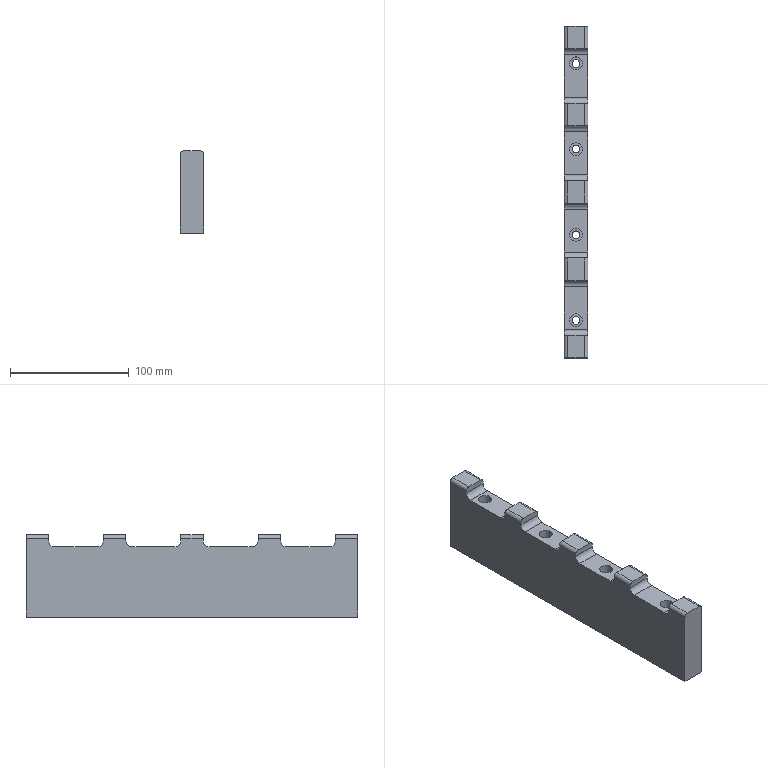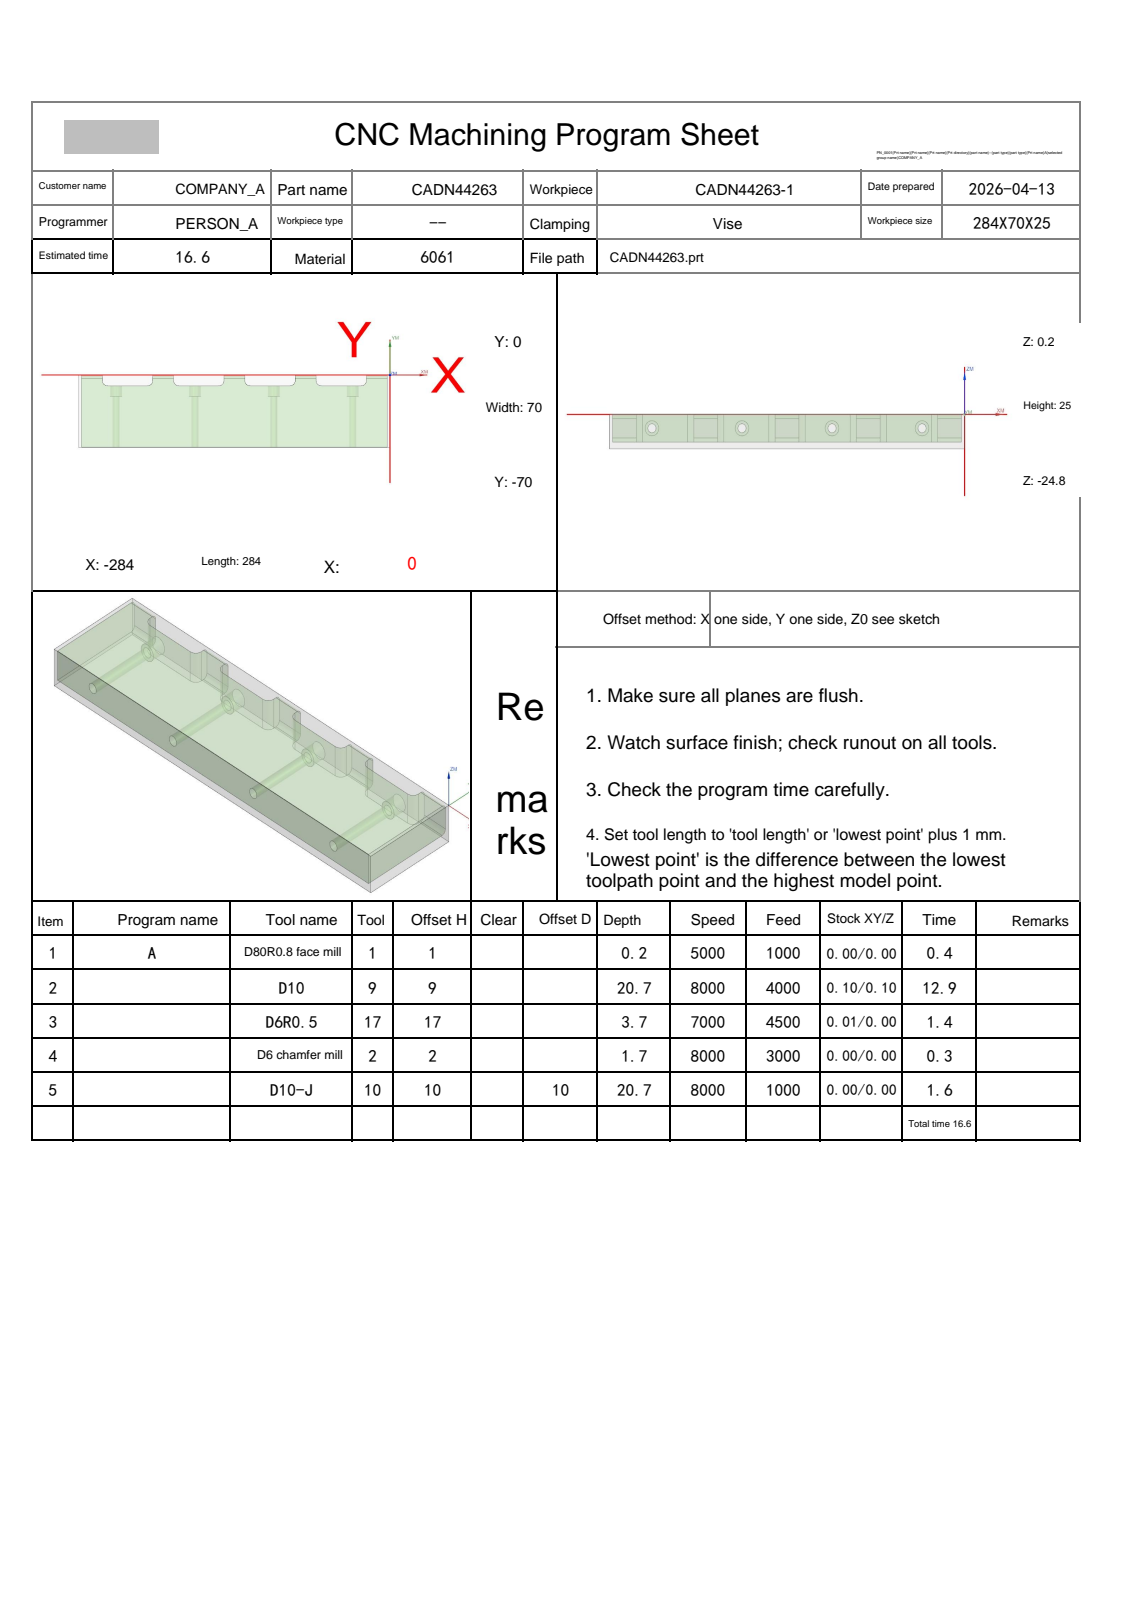NC program | NX | posted by the shop | part box 20 x 279 x 69 mm
Lines 7914 to 9859 of 9859:
N3 T17 M06
(D6R0.5  D=6. R=0.5 H=17 ce=0.01 di=0.00)
G00 G90 G54 X-27.305 Y-.497 M03 S7000
G43 H17 Z10.2
M08
Z.493
G01 Z-.007 F4500.
X-22.6 Y-.968
X-22.418 Y-.967
X-21.5 Y-.762
X-2.5
G03 X-1.496 Y-.906 I1.004 J3.433
G01 X-1.377 Y-.904
X-1.388 Y-.838 Z-.015
G03 X-2.5 Y-.667 I-1.295 J-4.708
G01 X-21.5
X-22.6 Y-.861
Y-.779 Z-.019
Y-.748 Z-.023
X-22.38 Y-.732
X-21.5 Y-.59
X-2.5
X-1.397 Y-.771
X-1.4 Y-.71 Z-.032
G03 X-2.5 Y-.521 I-3.068 J-14.528
G01 X-21.5
X-22.418 Y-.687
X-22.6 Y-.688
Y-.639 Z-.037
Y-.627 Z-.042
X-21.5 Y-.447
X-2.5
G02 X-1.4 Y-.653 I-2.113 J-14.314
G01 Y-.602 Z-.049
Y-.587 Z-.055
X-1.608 Y-.53
X-2.5 Y-.372
X-21.5
X-22.6 Y-.554
Y-.493 Z-.062
Y-.472 Z-.069
X-21.5 Y-.297
X-2.5
G02 X-1.4 Y-.511 I-.298 J-4.464
G01 Y-.425 Z-.086
X-2.5 Y-.221
X-21.5
X-22.6 Y-.382
Y-.345 Z-.095
Y-.314 Z-.104
X-21.5 Y-.143
X-2.5
X-1.4 Y-.343
Y-.304 Z-.114
Y-.258 Z-.125
X-2.5 Y-.063
X-21.5
X-22.6 Y-.235
Y-.189 Z-.137
Y-.148 Z-.148
X-21.5 Y.018
X-2.5
G02 X-1.4 Y-.164 I-.51 J-6.477
G01 Y-.114 Z-.161
Y-.062 Z-.174
X-1.576 Y-.054
X-1.673 Y-.027
X-2.5 Y.099
X-21.5
X-22.6 Y-.053
Y.003 Z-.188
Y.044 Z-.203
X-21.5 Y.184
X-2.5
G03 X-1.399 Y.042 I9.198 J66.835
G01 Y.095 Z-.219
X-1.398 Y.144 Z-.235
G02 X-2.5 Y.27 I.451 J8.779
G01 X-21.5
X-22.6 Y.142
Y.186 Z-.252
Y.225 Z-.269
X-21.5 Y.356
X-2.5
X-1.912 Y.291
X-1.826 Y.267
X-1.399 Y.227
X-1.4 Y.272 Z-.288
Y.314 Z-.306
X-2.5 Y.442
X-21.5
X-22.418 Y.317
X-22.6 Y.314
Y.354 Z-.321
Y.384 Z-.337
G03 X-21.5 Y.507 I-11.808 J110.237
G01 X-2.5
G03 X-1.4 Y.383 I2.105 J13.666
G01 Y.436 Z-.355
Y.467 Z-.374
G02 X-2.5 Y.584 I.826 J12.997
G01 X-21.5
X-22.418 Y.478
X-22.6 Y.47
Y.532 Z-.396
Y.566 Z-.418
X-22.418 Y.572
X-21.5 Y.669
X-2.5
G03 X-1.4 Y.567 I1.918 J14.664
G01 Y.619 Z-.442
Y.661 Z-.465
G02 X-2.5 Y.753 I.149 J8.39
G01 X-21.5
X-22.418 Y.662
X-22.6 Y.66
Y.702 Z-.49
Y.74 Z-.515
X-22.418 Y.743
X-21.5 Y.837
X-2.5
G03 X-1.4 Y.742 I1.224 J7.766
G01 Y.785 Z-.54
Y.826 Z-.566
G02 X-2.5 Y.918 I.174 J8.658
G01 X-21.5
X-22.418 Y.827
X-22.6 Y.824
Y.868 Z-.591
Y.907 Z-.617
X-22.418 Y.91
X-21.5 Y.995
X-2.5
G02 X-1.758 Y.91 I-.148 J-4.592
G01 X-1.4 Y.909
Y.953 Z-.644
Y.99 Z-.67
G02 X-2.5 Y1.069 I.078 J8.763
G01 X-21.5
X-22.418 Y.991
X-22.6 Y.989
Y1.037 Z-.699
Y1.062 Z-.729
X-22.418 Y1.064
X-21.5 Y1.148
X-2.5
G03 X-1.4 Y1.063 I1.15 J7.772
G01 Y1.114 Z-.759
Y1.139 Z-.79
G02 X-2.5 Y1.225 I.077 J8.113
G01 X-21.5
G02 X-22.6 Y1.138 I-1.349 J10.062
G01 Y1.187 Z-.822
Y1.216 Z-.853
G03 X-21.5 Y1.3 I-.451 J13.214
G01 X-2.5
G03 X-1.4 Y1.218 I1.277 J9.723
G01 Y1.263 Z-.886
Y1.3 Z-.919
G02 X-2.5 Y1.374 I.219 J11.451
G01 X-21.5
G02 X-22.6 Y1.298 I-1.629 J15.613
G01 Y1.341 Z-.952
Y1.374 Z-.986
G03 X-21.5 Y1.445 I-.337 J13.725
G01 X-2.5
G03 X-1.4 Y1.376 I1.224 J10.625
G01 X-1.399 Y1.419 Z-1.021
Y1.453 Z-1.056
G02 X-2.5 Y1.515 I.127 J11.964
G01 X-21.5
G02 X-22.6 Y1.451 I-1.481 J15.85
G01 Y1.489 Z-1.092
Y1.52 Z-1.128
G03 X-21.5 Y1.584 I-.16 J12.289
G01 X-2.5
G03 X-1.399 Y1.521 I1.136 J10.344
G01 Y1.554 Z-1.165
X-1.4 Y1.585 Z-1.202
G02 X-2.5 Y1.65 I.093 J10.893
G01 X-21.5
G03 X-22.073 Y1.596 I.041 J-3.531
G01 X-22.6 Y1.583
Y1.618 Z-1.24
Y1.648 Z-1.278
X-22.073 Y1.661
G02 X-21.5 Y1.714 I.679 J-4.208
G01 X-2.5
G03 X-1.4 Y1.649 I1.189 J10.851
G01 Y1.683 Z-1.316
Y1.713 Z-1.355
G02 X-2.5 Y1.776 I.065 J10.868
G01 X-21.5
G02 X-22.6 Y1.712 I-1.413 J14.76
G01 Y1.75 Z-1.395
Y1.777 Z-1.434
G03 X-21.5 Y1.836 I-.604 J21.629
G01 X-2.5
G03 X-1.399 Y1.779 I1.204 J12.62
G01 Y1.81 Z-1.475
Y1.84 Z-1.516
X-1.42
G02 X-2.5 Y1.893 I0.0 J11.063
G01 X-21.5
G02 X-22.6 Y1.839 I-1.187 J12.876
G01 Y1.867 Z-1.557
Y1.89 Z-1.598
X-22.073 Y1.9
X-21.5 Y1.948
X-2.5
G03 X-1.412 Y1.891 I1.088 J10.306
G01 X-1.399
Y1.918 Z-1.641
X-1.4 Y1.943 Z-1.683
X-1.562 Y1.938
G02 X-1.773 Y1.946 I0.0 J2.647
G01 X-2.447 Y2.
X-2.5 Y2.001
X-21.5
G03 X-22.073 Y1.952 I.057 J-4.043
G01 X-22.6 Y1.941
Y1.97 Z-1.726
Y1.996 Z-1.769
X-22.073 Y2.005
G02 X-21.5 Y2.052 I.847 J-6.832
G01 X-2.5
G03 X-1.446 Y1.996 I1.054 J9.941
G01 X-1.4
Y2.023 Z-1.812
X-1.399 Y2.049 Z-1.856
X-1.52 Y2.048
G02 X-2.5 Y2.1 I0.0 J9.293
G01 X-21.5
G02 X-22.6 Y2.047 I-1.179 J13.117
G01 Y2.073 Z-1.9
Y2.096 Z-1.945
G03 X-21.5 Y2.145 I-.089 J14.098
G01 X-2.5
G03 X-1.528 Y2.096 I.972 J9.5
G01 X-1.399 Y2.097
Y2.118 Z-1.99
Y2.136 Z-2.035
X-1.411
G02 X-2.5 Y2.189 I0.0 J11.318
G01 X-21.5
G03 X-22.073 Y2.144 I.096 J-4.959
G01 X-22.6 Y2.135
Y2.157 Z-2.08
Y2.174 Z-2.126
X-22.073 Y2.183
G02 X-21.5 Y2.229 I.696 J-5.119
G01 X-2.5
G03 X-1.42 Y2.175 I1.08 J10.819
G01 X-1.399
Y2.195 Z-2.172
Y2.214 Z-2.218
X-1.403
G02 X-2.5 Y2.267 I0.0 J11.287
G01 X-21.5
G03 X-22.073 Y2.222 I.075 J-4.597
G01 X-22.6 Y2.212
Y2.234 Z-2.265
Y2.251 Z-2.312
X-22.073 Y2.259
G02 X-21.5 Y2.302 I.781 J-6.53
G01 X-2.5
G03 X-1.458 Y2.252 I1.041 J10.8
G01 X-1.399
Y2.271 Z-2.359
Y2.291 Z-2.406
X-1.511 Y2.29
G02 X-2.5 Y2.335 I0.0 J10.989
G01 X-21.5
G03 X-22.073 Y2.291 I.123 J-5.442
G01 X-22.6 Y2.289
Y2.308 Z-2.454
Y2.316 Z-2.502
X-22.073 Y2.324
X-21.5 Y2.365
X-2.5
G03 X-1.448 Y2.318 I1.052 J11.969
G01 X-1.4 Y2.319
Y2.333 Z-2.55
Y2.346 Z-2.598
X-1.538 Y2.345
G02 X-2.5 Y2.392 I0.0 J9.984
G01 X-21.5
G02 X-22.604 Y2.343 I-1.132 J13.014
G01 Y2.354 Z-2.646
Y2.366 Z-2.695
G03 X-21.5 Y2.416 I-.184 J16.282
G01 X-2.5
G03 X-1.557 Y2.371 I.943 J9.825
G01 X-1.405 Y2.372
X-1.404 Y2.385 Z-2.744
Y2.398 Z-2.792
X-1.564 Y2.397
G02 X-2.5 Y2.438 I0.0 J10.791
G01 X-21.5
G02 X-22.604 Y2.39 I-1.539 J22.701
G01 X-22.605 Y2.401 Z-2.841
Y2.413 Z-2.891
G03 X-21.5 Y2.457 I-.624 J29.922
G01 X-2.5
G03 X-1.538 Y2.424 I.962 J14.016
G01 X-1.402
Y2.431 Z-2.94
X-1.401 Y2.444 Z-2.989
X-1.586 Y2.443
G02 X-2.5 Y2.473 I0.0 J14.194
G01 X-21.5
G02 X-22.605 Y2.434 I-1.958 J40.051
G01 Y2.444 Z-3.039
Y2.454 Z-3.088
X-21.5 Y2.486
X-2.5
G03 X-1.634 Y2.461 I.866 J14.975
X-1.4 Y2.463 I0.0 J15.
G01 Y2.471 Z-3.138
Y2.476 Z-3.188
G02 X-1.643 Y2.475 I-.243 J17.246
X-2.5 Y2.496 I0.0 J17.248
G01 X-21.5
G02 X-22.459 Y2.473 I-.959 J19.531
G01 X-22.6
X-22.595 Y2.483 Z-3.266
X-22.411 Y2.482
G03 X-21.5 Y2.502 I0.0 J20.891
G01 X-2.5
X-2.447 Y2.498
X-1.399 Y2.486
Y2.495 Z-3.344
X-2.5 Y2.507
X-21.5
G02 X-22.383 Y2.492 I-.883 J27.323
G01 X-22.595 Y2.493
Y2.503 Z-3.422
X-21.5 Y2.509
X-2.5
X-1.398 Y2.504
Y2.509 Z-3.5
X-22.595 Y2.51
G00 Z10.2
X-92.277 Y-.467
Z.493
G01 Z-.007
X-87.6 Y-.968
X-87.382 Y-.967
X-86.5 Y-.762
X-67.5
X-66.618 Y-.967
X-66.41 Y-.927
X-66.403 Y-.862 Z-.011
X-66.402 Y-.849 Z-.015
X-67.31 Y-.693
X-67.5 Y-.667
X-86.5
G02 X-87.6 Y-.86 I-11.743 J63.548
G01 Y-.779 Z-.019
Y-.748 Z-.023
X-86.5 Y-.59
X-67.5
X-66.398 Y-.768
X-66.4 Y-.71 Z-.032
X-66.613 Y-.682
X-67.5 Y-.521
X-86.5
X-87.382 Y-.687
X-87.6 Y-.688
Y-.639 Z-.037
Y-.625 Z-.042
X-87.382 Y-.623
X-86.5 Y-.447
X-67.5
X-66.609 Y-.607
X-66.4 Y-.653
Y-.602 Z-.049
Y-.585 Z-.055
X-66.596 Y-.545
X-67.5 Y-.372
X-86.5
X-87.382 Y-.549
X-87.6 Y-.552
Y-.493 Z-.062
Y-.469 Z-.069
X-86.5 Y-.297
X-67.5
G02 X-66.4 Y-.508 I-1.243 J-9.475
G01 Y-.457 Z-.077
Y-.419 Z-.086
X-66.566 Y-.393
X-67.5 Y-.221
X-86.5
X-87.6 Y-.38
Y-.345 Z-.095
Y-.311 Z-.104
X-86.5 Y-.143
X-67.5
X-66.445 Y-.33
Y-.302 Z-.114
Y-.247 Z-.125
X-67.5 Y-.063
X-86.5
X-87.6 Y-.232
Y-.189 Z-.137
Y-.145 Z-.148
X-86.5 Y.018
X-67.5
X-67.31 Y.003
X-66.445 Y-.154
X-66.439 Y-.114 Z-.161
X-66.43 Y-.057 Z-.174
X-67.5 Y.099
X-86.5
X-87.6 Y-.05
Y.003 Z-.188
Y.046 Z-.203
X-87.382 Y.05
X-86.5 Y.184
X-67.5
X-66.618 Y.05
X-66.399 Y.043
X-66.4 Y.096 Z-.219
Y.143 Z-.235
X-67.5 Y.27
X-86.5
X-87.382 Y.145
X-87.6 Y.143
Y.186 Z-.252
Y.226 Z-.269
X-87.382 Y.228
X-86.5 Y.356
X-67.5
X-66.4 Y.226
Y.272 Z-.288
Y.313 Z-.306
X-66.618 Y.315
X-67.5 Y.442
X-86.5
X-87.382 Y.317
X-87.6 Y.314
Y.354 Z-.321
Y.384 Z-.337
G03 X-86.5 Y.507 I-11.318 J105.893
G01 X-67.5
X-66.618 Y.384
X-66.4 Y.382
Y.436 Z-.355
Y.466 Z-.374
X-67.5 Y.584
X-86.5
X-87.382 Y.478
X-87.6 Y.47
Y.533 Z-.396
Y.567 Z-.418
X-87.131 Y.6
X-87.036 Y.617
G02 X-86.5 Y.669 I.598 J-3.336
G01 X-67.5
X-66.4 Y.565
Y.619 Z-.442
Y.66 Z-.465
X-66.618 Y.662
X-67.5 Y.753
X-86.5
G02 X-87.6 Y.66 I-1.695 J13.465
G01 Y.702 Z-.49
Y.741 Z-.515
G03 X-86.5 Y.837 I-.518 J12.298
G01 X-67.5
G02 X-66.792 Y.747 I-.042 J-3.181
G01 X-66.4 Y.741
Y.785 Z-.54
Y.825 Z-.566
X-66.618 Y.827
X-67.5 Y.918
X-86.5
G02 X-87.6 Y.825 I-1.556 J11.791
G01 Y.868 Z-.591
Y.908 Z-.617
X-87.382 Y.91
X-86.5 Y.995
X-67.5
X-66.4 Y.908
Y.953 Z-.644
Y.99 Z-.67
X-66.618 Y.991
X-67.5 Y1.069
X-86.5
G02 X-87.6 Y.99 I-1.409 J11.774
G01 Y1.037 Z-.699
Y1.063 Z-.729
G03 X-86.5 Y1.148 I-.234 J10.139
G01 X-67.5
X-66.618 Y1.064
X-66.4 Y1.063
Y1.114 Z-.759
Y1.138 Z-.79
X-66.618 Y1.14
X-67.5 Y1.225
X-86.5
G02 X-87.6 Y1.138 I-1.321 J9.774
G01 Y1.187 Z-.822
Y1.217 Z-.853
X-87.455 Y1.21
X-87.295 Y1.219
X-86.5 Y1.3
X-67.5
X-66.618 Y1.219
X-66.4 Y1.217
Y1.263 Z-.886
Y1.298 Z-.919
X-66.618 Y1.3
X-67.5 Y1.374
X-86.5
X-87.036 Y1.323
X-87.12 Y1.314
X-87.6 Y1.298
Y1.341 Z-.952
Y1.375 Z-.986
X-87.382 Y1.377
X-86.5 Y1.445
X-67.5
X-66.618 Y1.377
X-66.4 Y1.375
Y1.419 Z-1.021
Y1.452 Z-1.056
X-66.618 Y1.454
X-67.5 Y1.515
X-86.5
X-87.382 Y1.454
X-87.6 Y1.452
Y1.489 Z-1.092
Y1.521 Z-1.128
G03 X-86.5 Y1.584 I-.106 J11.464
G01 X-67.5
G03 X-66.4 Y1.521 I1.206 J11.401
G01 Y1.554 Z-1.165
Y1.584 Z-1.202
X-66.964 Y1.6
G03 X-67.5 Y1.65 I-.558 J-3.082
G01 X-86.5
G03 X-87.036 Y1.6 I.021 J-3.132
G01 X-87.6 Y1.584
Y1.618 Z-1.24
Y1.648 Z-1.278
G03 X-86.5 Y1.714 I-.353 J15.186
G01 X-67.5
G03 X-66.4 Y1.648 I1.453 J15.12
G01 Y1.683 Z-1.316
Y1.712 Z-1.355
G02 X-67.5 Y1.776 I.249 J13.86
G01 X-86.5
G02 X-87.6 Y1.712 I-1.349 J13.797
G01 Y1.75 Z-1.395
Y1.777 Z-1.434
G03 X-86.5 Y1.836 I-.651 J22.793
G01 X-67.5
G03 X-66.4 Y1.777 I1.752 J22.735
G01 Y1.81 Z-1.475
Y1.839 Z-1.516
G02 X-67.5 Y1.893 I.06 J12.531
G01 X-86.5
G02 X-87.6 Y1.839 I-1.16 J12.478
G01 Y1.867 Z-1.557
Y1.89 Z-1.598
G03 X-86.5 Y1.948 I-.169 J13.623
G01 X-67.5
G03 X-66.4 Y1.89 I1.269 J13.564
G01 Y1.918 Z-1.641
Y1.942 Z-1.683
X-66.964 Y1.955
G03 X-67.5 Y2.001 I-.55 J-3.271
G01 X-86.5
G03 X-87.036 Y1.955 I.02 J-3.386
G01 X-87.6 Y1.942
Y1.97 Z-1.726
Y1.996 Z-1.769
G03 X-86.5 Y2.052 I-.175 J14.347
G01 X-67.5
G03 X-66.4 Y1.996 I1.275 J14.292
G01 Y2.023 Z-1.812
Y2.048 Z-1.856
G02 X-67.5 Y2.1 I.069 J13.12
G01 X-86.5
G02 X-87.6 Y2.048 I-1.169 J13.068
G01 Y2.073 Z-1.9
Y2.096 Z-1.945
G03 X-86.5 Y2.145 I-.103 J14.555
G01 X-67.5
G03 X-66.4 Y2.096 I1.203 J14.506
G01 Y2.118 Z-1.99
Y2.135 Z-2.035
X-66.964 Y2.147
G03 X-67.5 Y2.189 I-.605 J-4.327
G01 X-86.5
G03 X-87.036 Y2.147 I.069 J-4.369
G01 X-87.6 Y2.135
Y2.157 Z-2.08
Y2.174 Z-2.126
X-87.036 Y2.186
G02 X-86.5 Y2.229 I.622 J-4.418
G01 X-67.5
G02 X-66.964 Y2.186 I-.086 J-4.461
G01 X-66.4 Y2.174
Y2.195 Z-2.172
Y2.213 Z-2.218
X-66.964 Y2.225
G03 X-67.5 Y2.267 I-.59 J-4.056
G01 X-86.5
G03 X-87.036 Y2.225 I.054 J-4.098
G01 X-87.6 Y2.213
Y2.234 Z-2.265
Y2.251 Z-2.312
X-87.036 Y2.261
G02 X-86.5 Y2.302 I.689 J-5.53
G01 X-67.5
G02 X-66.964 Y2.263 I-.182 J-6.232
G01 X-66.4 Y2.251
Y2.271 Z-2.359
Y2.29 Z-2.406
X-66.964 Y2.3
G03 X-67.5 Y2.335 I-.669 J-6.159
G01 X-86.5
X-86.69 Y2.328
G02 X-87.361 Y2.284 I-.671 J5.154
X-87.6 Y2.29 I0.0 J5.198
G01 Y2.307 Z-2.454
Y2.316 Z-2.502
G03 X-86.5 Y2.365 I-.147 J15.87
G01 X-67.5
G03 X-66.4 Y2.318 I1.19 J15.04
G01 X-66.398 Y2.333 Z-2.55
X-66.397 Y2.346 Z-2.598
X-66.453
G02 X-67.5 Y2.392 I0.0 J12.019
G01 X-86.5
G02 X-87.603 Y2.343 I-1.135 J13.09
G01 Y2.354 Z-2.646
Y2.366 Z-2.695
G03 X-86.5 Y2.416 I-.267 J18.114
G01 X-67.5
G02 X-66.964 Y2.378 I-.19 J-6.461
G01 X-66.397 Y2.372
Y2.385 Z-2.744
Y2.398 Z-2.792
X-66.964 Y2.403
X-67.5 Y2.438
X-86.5
G02 X-87.603 Y2.39 I-1.534 J22.69
G01 Y2.401 Z-2.841
Y2.414 Z-2.891
G03 X-86.5 Y2.457 I-.475 J26.586
G01 X-67.5
G03 X-66.565 Y2.423 I.935 J13.098
G01 X-66.397 Y2.424
Y2.431 Z-2.94
X-66.396 Y2.443 Z-2.989
X-66.571 Y2.442
G02 X-67.5 Y2.473 I0.0 J14.242
G01 X-86.5
G02 X-87.603 Y2.435 I-1.619 J31.516
G01 X-87.604 Y2.444 Z-3.039
Y2.455 Z-3.088
X-86.69 Y2.476
X-86.5 Y2.486
X-67.5
G03 X-66.642 Y2.46 I.858 J14.468
X-66.396 Y2.462 I0.0 J14.494
G01 Y2.466 Z-3.138
Y2.476 Z-3.188
X-67.31 Y2.484
X-67.5 Y2.496
X-86.5
X-86.69 Y2.484
X-87.604 Y2.472
Y2.479 Z-3.227
Y2.482 Z-3.266
X-86.69 Y2.491
X-86.5 Y2.502
X-67.5
X-67.31 Y2.491
X-66.396 Y2.485
Y2.494 Z-3.344
X-67.31 Y2.498
X-67.5 Y2.507
X-86.5
X-86.69 Y2.498
X-87.604 Y2.492
Y2.498 Z-3.383
Y2.503 Z-3.422
X-86.69 Y2.505
X-86.5 Y2.509
X-67.5
X-67.31 Y2.505
X-66.396 Y2.503
Y2.509 Z-3.5
X-87.604
G00 Z10.2
X-157.272 Y-.463
Z.493
G01 Z-.007
X-152.6 Y-.968
X-152.384
X-151.5 Y-.762
X-132.5
X-131.616 Y-.968
X-131.41 Y-.928
X-131.403 Y-.862 Z-.011
X-131.402 Y-.849 Z-.015
G02 X-132.5 Y-.667 I3.048 J21.767
G01 X-151.5
G02 X-152.6 Y-.86 I-11.751 J63.549
G01 Y-.779 Z-.019
Y-.747 Z-.023
X-151.5 Y-.59
X-132.5
X-131.398 Y-.768
X-131.4 Y-.71 Z-.032
X-131.611 Y-.682
X-132.5 Y-.521
X-151.5
X-152.384 Y-.687
X-152.6 Y-.688
Y-.639 Z-.037
Y-.626 Z-.042
X-152.384 Y-.624
X-151.5 Y-.447
X-132.5
X-131.608 Y-.608
X-131.4 Y-.652
Y-.602 Z-.049
Y-.584 Z-.055
X-131.595 Y-.545
X-132.5 Y-.372
X-151.5
X-152.384 Y-.55
X-152.6 Y-.552
Y-.493 Z-.062
Y-.469 Z-.069
X-151.5 Y-.297
X-132.5
G02 X-131.4 Y-.506 I-.939 J-7.967
G01 Y-.458 Z-.077
Y-.416 Z-.086
X-131.564 Y-.394
X-132.5 Y-.221
X-151.5
X-152.6 Y-.381
Y-.345 Z-.095
Y-.311 Z-.104
X-151.5 Y-.143
X-132.5
X-131.443 Y-.33
Y-.302 Z-.114
Y-.247 Z-.125
X-132.5 Y-.063
X-151.5
X-152.6 Y-.233
Y-.189 Z-.137
Y-.145 Z-.148
X-151.5 Y.018
X-132.5
X-132.308 Y.003
X-131.443 Y-.154
X-131.437 Y-.114 Z-.161
X-131.428 Y-.058 Z-.174
X-132.5 Y.099
X-151.5
X-152.6 Y-.05
Y.003 Z-.188
Y.046 Z-.203
X-152.384 Y.05
X-151.5 Y.184
X-132.5
X-131.616 Y.05
X-131.4 Y.043
Y.105 Z-.219
Y.143 Z-.235
X-132.5 Y.27
X-151.5
X-152.384 Y.145
X-152.6 Y.143
Y.186 Z-.252
Y.226 Z-.269
X-152.384 Y.228
X-151.5 Y.356
X-132.5
X-131.4 Y.226
Y.272 Z-.288
Y.313 Z-.306
X-131.616 Y.315
X-132.5 Y.442
X-151.5
X-152.384 Y.317
X-152.6 Y.314
Y.354 Z-.321
Y.384 Z-.337
G03 X-151.5 Y.507 I-11.356 J106.243
G01 X-132.5
X-131.616 Y.384
X-131.4 Y.382
Y.436 Z-.355
Y.466 Z-.374
X-132.5 Y.584
X-151.5
X-152.384 Y.478
X-152.6 Y.47
Y.532 Z-.396
Y.567 Z-.418
X-152.132 Y.599
X-152.038 Y.616
G02 X-151.5 Y.669 I.601 J-3.358
G01 X-132.5
X-131.4 Y.566
Y.619 Z-.442
Y.66 Z-.465
X-131.616 Y.662
X-132.5 Y.753
X-151.5
G02 X-152.6 Y.66 I-1.692 J13.423
G01 Y.702 Z-.49
Y.741 Z-.515
G03 X-151.5 Y.837 I-.521 J12.33
G01 X-132.5
G02 X-131.791 Y.747 I-.043 J-3.197
G01 X-131.4 Y.741
Y.785 Z-.54
Y.825 Z-.566
X-131.616 Y.827
X-132.5 Y.918
X-151.5
G02 X-152.6 Y.825 I-1.559 J11.819
G01 Y.868 Z-.591
Y.908 Z-.617
X-152.384 Y.91
X-151.5 Y.995
X-132.5
X-131.4 Y.908
Y.953 Z-.644
Y.989 Z-.67
X-131.616 Y.991
X-132.5 Y1.069
X-151.5
G02 X-152.6 Y.989 I-1.413 J11.802
G01 Y1.037 Z-.699
Y1.062 Z-.729
G03 X-151.5 Y1.148 I-.236 J10.156
G01 X-132.5
X-131.616 Y1.064
X-131.4 Y1.062
Y1.114 Z-.759
Y1.138 Z-.79
X-131.616 Y1.14
X-132.5 Y1.225
X-151.5
G02 X-152.6 Y1.138 I-1.324 J9.804
G01 Y1.187 Z-.822
Y1.217 Z-.853
X-152.46 Y1.212
G03 X-152.25 Y1.223 I0.0 J2.061
G01 X-151.5 Y1.3
X-132.5
X-131.616 Y1.219
X-131.4 Y1.217
Y1.263 Z-.886
Y1.298 Z-.919
X-131.616 Y1.3
X-132.5 Y1.374
X-151.5
X-152.038 Y1.322
X-152.126 Y1.313
X-152.6 Y1.298
Y1.341 Z-.952
Y1.375 Z-.986
X-152.384 Y1.377
X-151.5 Y1.445
X-132.5
X-131.616 Y1.377
X-131.4 Y1.375
Y1.419 Z-1.021
Y1.452 Z-1.056
X-131.616 Y1.454
X-132.5 Y1.515
X-151.5
X-152.384 Y1.454
X-152.6 Y1.452
Y1.489 Z-1.092
Y1.52 Z-1.128
G03 X-151.5 Y1.584 I-.108 J11.494
G01 X-132.5
G03 X-131.4 Y1.52 I1.208 J11.431
G01 Y1.554 Z-1.165
Y1.584 Z-1.202
X-131.962 Y1.6
G03 X-132.5 Y1.65 I-.559 J-3.085
G01 X-151.5
G03 X-152.038 Y1.6 I.021 J-3.135
G01 X-152.6 Y1.584
Y1.618 Z-1.24
Y1.648 Z-1.278
G03 X-151.5 Y1.714 I-.356 J15.217
G01 X-132.5
G03 X-131.4 Y1.648 I1.456 J15.152
G01 Y1.683 Z-1.316
Y1.712 Z-1.355
G02 X-132.5 Y1.776 I.253 J13.933
G01 X-151.5
G02 X-152.6 Y1.712 I-1.353 J13.869
G01 Y1.75 Z-1.395
Y1.778 Z-1.434
G03 X-151.5 Y1.836 I-.659 J22.958
G01 X-132.5
G03 X-131.4 Y1.778 I1.759 J22.902
G01 Y1.81 Z-1.475
Y1.839 Z-1.516
G02 X-132.5 Y1.893 I.061 J12.531
G01 X-151.5
G02 X-152.6 Y1.839 I-1.161 J12.477
G01 Y1.867 Z-1.557
Y1.89 Z-1.598
G03 X-151.5 Y1.948 I-.174 J13.705
G01 X-132.5
G03 X-131.4 Y1.89 I1.274 J13.647
G01 Y1.918 Z-1.641
Y1.942 Z-1.683
X-131.962 Y1.955
G03 X-132.5 Y2.001 I-.551 J-3.272
G01 X-151.5
G03 X-152.038 Y1.955 I.017 J-3.362
G01 X-152.6 Y1.942
Y1.97 Z-1.726
Y1.996 Z-1.769
G03 X-151.5 Y2.052 I-.189 J14.503
G01 X-132.5
G03 X-131.4 Y1.996 I1.288 J14.447
G01 Y2.023 Z-1.812
Y2.048 Z-1.856
G02 X-132.5 Y2.1 I.07 J13.129
G01 X-151.5
G02 X-152.6 Y2.048 I-1.17 J13.077
G01 Y2.073 Z-1.9
Y2.096 Z-1.945
G03 X-151.5 Y2.145 I-.111 J14.702
G01 X-132.5
G03 X-131.4 Y2.096 I1.211 J14.652
G01 Y2.12 Z-1.99
Y2.135 Z-2.035
X-131.962 Y2.147
G03 X-132.5 Y2.189 I-.608 J-4.36
G01 X-151.5
G03 X-152.038 Y2.147 I.07 J-4.402
G01 X-152.6 Y2.135
Y2.157 Z-2.08
Y2.174 Z-2.126
X-152.038 Y2.186
G02 X-151.5 Y2.229 I.624 J-4.432
G01 X-132.5
G02 X-131.962 Y2.186 I-.086 J-4.475
G01 X-131.4 Y2.174
Y2.195 Z-2.172
Y2.213 Z-2.218
X-131.962 Y2.224
G03 X-132.5 Y2.267 I-.594 J-4.092
G01 X-151.5
G03 X-152.038 Y2.224 I.056 J-4.134
G01 X-152.6 Y2.213
Y2.234 Z-2.265
Y2.251 Z-2.312
X-152.038 Y2.261
G02 X-151.5 Y2.302 I.691 J-5.54
G01 X-132.5
G02 X-131.962 Y2.263 I-.184 J-6.258
G01 X-131.4 Y2.251
Y2.271 Z-2.359
Y2.29 Z-2.406
X-131.962 Y2.3
G03 X-132.5 Y2.335 I-.668 J-6.118
G01 X-151.5
X-151.692 Y2.328
G02 X-152.36 Y2.284 I-.669 J5.13
X-152.6 Y2.29 I0.0 J5.174
G01 Y2.307 Z-2.454
Y2.316 Z-2.502
G03 X-151.5 Y2.365 I-.142 J15.739
G01 X-132.5
G03 X-131.4 Y2.318 I1.186 J14.917
G01 Y2.333 Z-2.55
Y2.346 Z-2.598
X-131.457
G02 X-132.5 Y2.392 I0.0 J11.927
G01 X-151.5
G02 X-152.6 Y2.343 I-1.132 J13.003
G01 Y2.354 Z-2.646
Y2.366 Z-2.695
G03 X-151.5 Y2.416 I-.26 J17.894
G01 X-132.5
G02 X-131.962 Y2.378 I-.199 J-6.597
G01 X-131.4 Y2.372
Y2.385 Z-2.744
Y2.398 Z-2.792
X-131.962 Y2.403
G03 X-132.5 Y2.438 I-.695 J-6.615
G01 X-151.5
G02 X-152.6 Y2.39 I-1.541 J22.828
G01 Y2.402 Z-2.841
Y2.414 Z-2.891
X-152.384 Y2.418
X-151.5 Y2.457
X-132.5
G03 X-131.514 Y2.422 I.986 J14.218
G01 X-131.401 Y2.423
X-131.4 Y2.437 Z-2.94
Y2.443 Z-2.989
X-131.572 Y2.442
G02 X-132.5 Y2.473 I0.0 J14.315
G01 X-151.5
X-152.384 Y2.439
X-152.6 Y2.435
Y2.445 Z-3.039
Y2.455 Z-3.088
X-151.692 Y2.475
X-151.5 Y2.486
X-132.5
G03 X-131.612 Y2.46 I.888 J15.263
X-131.4 Y2.461 I0.0 J15.289
G01 Y2.471 Z-3.138
Y2.475 Z-3.188
X-132.308 Y2.484
X-132.5 Y2.496
X-151.5
X-151.692 Y2.484
X-152.6 Y2.471
Y2.479 Z-3.227
Y2.482 Z-3.266
X-151.692 Y2.491
X-151.5 Y2.502
X-132.5
X-132.308 Y2.49
X-131.4 Y2.486
X-131.405 Y2.495 Z-3.344
X-131.411 Y2.493
X-132.308 Y2.497
X-132.5 Y2.507
X-151.5
X-151.692 Y2.497
X-152.589 Y2.492
X-152.6 Y2.494
X-152.595 Y2.502 Z-3.422
X-151.692 Y2.504
X-151.5 Y2.509
X-132.5
X-132.308 Y2.504
X-131.405 Y2.503
Y2.51 Z-3.5
X-152.595
G00 Z10.2
X-222.277 Y-.467
Z.493
G01 Z-.007
X-217.6 Y-.968
X-217.382 Y-.967
X-216.5 Y-.762
X-197.5
X-196.618 Y-.967
X-196.41 Y-.927
X-196.403 Y-.862 Z-.011
X-196.402 Y-.849 Z-.015
X-197.31 Y-.693
X-197.5 Y-.667
X-216.5
G02 X-217.6 Y-.86 I-11.743 J63.548
G01 Y-.779 Z-.019
Y-.748 Z-.023
X-216.5 Y-.59
X-197.5
X-196.398 Y-.768
X-196.4 Y-.71 Z-.032
X-196.613 Y-.682
X-197.5 Y-.521
X-216.5
X-217.382 Y-.687
X-217.6 Y-.688
Y-.639 Z-.037
Y-.625 Z-.042
X-217.382 Y-.623
X-216.5 Y-.447
X-197.5
X-196.609 Y-.607
X-196.4 Y-.653
Y-.602 Z-.049
Y-.585 Z-.055
X-196.596 Y-.545
X-197.5 Y-.372
X-216.5
X-217.382 Y-.549
X-217.6 Y-.552
Y-.493 Z-.062
Y-.469 Z-.069
X-216.5 Y-.297
X-197.5
G02 X-196.4 Y-.508 I-1.243 J-9.475
G01 Y-.457 Z-.077
Y-.419 Z-.086
X-196.566 Y-.393
X-197.5 Y-.221
X-216.5
X-217.6 Y-.38
Y-.345 Z-.095
Y-.311 Z-.104
X-216.5 Y-.143
X-197.5
X-196.445 Y-.33
Y-.302 Z-.114
Y-.247 Z-.125
X-197.5 Y-.063
X-216.5
X-217.6 Y-.232
Y-.189 Z-.137
Y-.145 Z-.148
X-216.5 Y.018
X-197.5
X-197.31 Y.003
X-196.445 Y-.154
X-196.439 Y-.114 Z-.161
X-196.43 Y-.057 Z-.174
X-197.5 Y.099
X-216.5
X-217.6 Y-.05
Y.003 Z-.188
Y.046 Z-.203
X-217.382 Y.05
X-216.5 Y.184
X-197.5
X-196.618 Y.05
X-196.399 Y.043
X-196.4 Y.096 Z-.219
Y.143 Z-.235
X-197.5 Y.27
X-216.5
X-217.382 Y.145
X-217.6 Y.143
Y.186 Z-.252
Y.226 Z-.269
X-217.382 Y.228
X-216.5 Y.356
X-197.5
X-196.4 Y.226
Y.272 Z-.288
Y.313 Z-.306
X-196.618 Y.315
X-197.5 Y.442
X-216.5
X-217.382 Y.317
X-217.6 Y.314
Y.354 Z-.321
Y.384 Z-.337
G03 X-216.5 Y.507 I-11.318 J105.893
G01 X-197.5
X-196.618 Y.384
X-196.4 Y.382
Y.436 Z-.355
Y.466 Z-.374
X-197.5 Y.584
X-216.5
X-217.382 Y.478
X-217.6 Y.47
Y.533 Z-.396
Y.567 Z-.418
X-217.131 Y.6
X-217.036 Y.617
G02 X-216.5 Y.669 I.598 J-3.336
G01 X-197.5
X-196.4 Y.565
Y.619 Z-.442
Y.66 Z-.465
X-196.618 Y.662
X-197.5 Y.753
X-216.5
G02 X-217.6 Y.66 I-1.695 J13.465
G01 Y.702 Z-.49
Y.741 Z-.515
G03 X-216.5 Y.837 I-.518 J12.298
G01 X-197.5
G02 X-196.792 Y.747 I-.042 J-3.181
G01 X-196.4 Y.741
Y.785 Z-.54
Y.825 Z-.566
X-196.618 Y.827
X-197.5 Y.918
X-216.5
G02 X-217.6 Y.825 I-1.556 J11.791
G01 Y.868 Z-.591
Y.908 Z-.617
X-217.382 Y.91
X-216.5 Y.995
X-197.5
X-196.4 Y.908
Y.953 Z-.644
Y.99 Z-.67
X-196.618 Y.991
X-197.5 Y1.069
X-216.5
G02 X-217.6 Y.99 I-1.409 J11.774
G01 Y1.037 Z-.699
Y1.063 Z-.729
G03 X-216.5 Y1.148 I-.234 J10.139
G01 X-197.5
X-196.618 Y1.064
X-196.4 Y1.063
Y1.114 Z-.759
Y1.138 Z-.79
X-196.618 Y1.14
X-197.5 Y1.225
X-216.5
G02 X-217.6 Y1.138 I-1.321 J9.774
G01 Y1.187 Z-.822
Y1.217 Z-.853
X-217.455 Y1.21
X-217.307 Y1.217
X-216.5 Y1.3
X-197.5
X-196.618 Y1.219
X-196.4 Y1.217
Y1.263 Z-.886
Y1.298 Z-.919
X-196.618 Y1.3
X-197.5 Y1.374
X-216.5
X-217.036 Y1.323
X-217.12 Y1.314
X-217.6 Y1.298
Y1.341 Z-.952
Y1.375 Z-.986
X-217.382 Y1.377
X-216.5 Y1.445
X-197.5
X-196.618 Y1.377
X-196.4 Y1.375
Y1.419 Z-1.021
Y1.452 Z-1.056
X-196.618 Y1.454
X-197.5 Y1.515
X-216.5
X-217.382 Y1.454
X-217.6 Y1.452
Y1.489 Z-1.092
Y1.521 Z-1.128
G03 X-216.5 Y1.584 I-.106 J11.464
G01 X-197.5
G03 X-196.4 Y1.521 I1.206 J11.401
G01 Y1.554 Z-1.165
Y1.584 Z-1.202
X-196.964 Y1.6
G03 X-197.5 Y1.65 I-.558 J-3.082
G01 X-216.5
G03 X-217.036 Y1.6 I.021 J-3.132
G01 X-217.6 Y1.584
Y1.618 Z-1.24
Y1.648 Z-1.278
G03 X-216.5 Y1.714 I-.353 J15.186
G01 X-197.5
G03 X-196.4 Y1.648 I1.453 J15.12
G01 Y1.683 Z-1.316
Y1.712 Z-1.355
G02 X-197.5 Y1.776 I.249 J13.86
G01 X-216.5
G02 X-217.6 Y1.712 I-1.349 J13.797
G01 Y1.75 Z-1.395
Y1.777 Z-1.434
G03 X-216.5 Y1.836 I-.651 J22.793
G01 X-197.5
G03 X-196.4 Y1.777 I1.752 J22.735
G01 Y1.81 Z-1.475
Y1.839 Z-1.516
G02 X-197.5 Y1.893 I.06 J12.531
G01 X-216.5
G02 X-217.6 Y1.839 I-1.16 J12.478
G01 Y1.867 Z-1.557
Y1.89 Z-1.598
G03 X-216.5 Y1.948 I-.169 J13.623
G01 X-197.5
G03 X-196.4 Y1.89 I1.269 J13.564
G01 Y1.918 Z-1.641
Y1.942 Z-1.683
X-196.964 Y1.955
G03 X-197.5 Y2.001 I-.55 J-3.271
G01 X-216.5
G03 X-217.036 Y1.955 I.02 J-3.386
G01 X-217.6 Y1.942
Y1.97 Z-1.726
Y1.996 Z-1.769
G03 X-216.5 Y2.052 I-.175 J14.347
G01 X-197.5
G03 X-196.4 Y1.996 I1.275 J14.292
G01 Y2.023 Z-1.812
Y2.048 Z-1.856
G02 X-197.5 Y2.1 I.069 J13.12
G01 X-216.5
G02 X-217.6 Y2.048 I-1.169 J13.068
G01 Y2.073 Z-1.9
Y2.096 Z-1.945
G03 X-216.5 Y2.145 I-.103 J14.555
G01 X-197.5
G03 X-196.4 Y2.096 I1.203 J14.506
G01 Y2.118 Z-1.99
Y2.135 Z-2.035
X-196.964 Y2.147
G03 X-197.5 Y2.189 I-.605 J-4.327
G01 X-216.5
G03 X-217.036 Y2.147 I.069 J-4.369
G01 X-217.6 Y2.135
Y2.157 Z-2.08
Y2.174 Z-2.126
X-217.036 Y2.186
G02 X-216.5 Y2.229 I.622 J-4.418
G01 X-197.5
G02 X-196.964 Y2.186 I-.086 J-4.461
G01 X-196.4 Y2.174
Y2.195 Z-2.172
Y2.213 Z-2.218
X-196.964 Y2.225
G03 X-197.5 Y2.267 I-.59 J-4.056
G01 X-216.5
G03 X-217.036 Y2.225 I.054 J-4.098
G01 X-217.6 Y2.213
Y2.234 Z-2.265
Y2.251 Z-2.312
X-217.036 Y2.261
G02 X-216.5 Y2.302 I.689 J-5.53
G01 X-197.5
G02 X-196.964 Y2.263 I-.182 J-6.232
G01 X-196.4 Y2.251
Y2.271 Z-2.359
Y2.29 Z-2.406
X-196.964 Y2.3
G03 X-197.5 Y2.335 I-.669 J-6.159
G01 X-216.5
X-216.69 Y2.328
G02 X-217.361 Y2.284 I-.671 J5.154
X-217.6 Y2.29 I0.0 J5.198
G01 Y2.307 Z-2.454
Y2.316 Z-2.502
G03 X-216.5 Y2.365 I-.147 J15.87
G01 X-197.5
G03 X-196.4 Y2.318 I1.19 J15.04
G01 X-196.398 Y2.333 Z-2.55
X-196.397 Y2.346 Z-2.598
X-196.453
G02 X-197.5 Y2.392 I0.0 J12.019
G01 X-216.5
G02 X-217.603 Y2.343 I-1.135 J13.09
G01 Y2.354 Z-2.646
Y2.366 Z-2.695
G03 X-216.5 Y2.416 I-.267 J18.114
G01 X-197.5
G02 X-196.964 Y2.378 I-.19 J-6.461
G01 X-196.397 Y2.372
Y2.385 Z-2.744
Y2.398 Z-2.792
X-196.964 Y2.403
X-197.5 Y2.438
X-216.5
G02 X-217.603 Y2.39 I-1.534 J22.69
G01 Y2.401 Z-2.841
Y2.414 Z-2.891
G03 X-216.5 Y2.457 I-.475 J26.586
G01 X-197.5
G03 X-196.565 Y2.423 I.935 J13.098
G01 X-196.397 Y2.424
Y2.431 Z-2.94
X-196.396 Y2.443 Z-2.989
X-196.571 Y2.442
G02 X-197.5 Y2.473 I0.0 J14.242
G01 X-216.5
G02 X-217.603 Y2.435 I-1.619 J31.516
G01 X-217.604 Y2.444 Z-3.039
Y2.455 Z-3.088
X-216.69 Y2.476
X-216.5 Y2.486
X-197.5
G03 X-196.642 Y2.46 I.858 J14.468
X-196.396 Y2.462 I0.0 J14.494
G01 Y2.466 Z-3.138
Y2.476 Z-3.188
X-197.31 Y2.484
X-197.5 Y2.496
X-216.5
X-216.69 Y2.484
X-217.604 Y2.472
Y2.479 Z-3.227
Y2.482 Z-3.266
X-216.69 Y2.491
X-216.5 Y2.502
X-197.5
X-197.31 Y2.491
X-196.396 Y2.485
Y2.494 Z-3.344
X-197.31 Y2.498
X-197.5 Y2.507
X-216.5
X-216.69 Y2.498
X-217.604 Y2.492
Y2.498 Z-3.383
Y2.503 Z-3.422
X-216.69 Y2.505
X-216.5 Y2.509
X-197.5
X-197.31 Y2.505
X-196.396 Y2.503
Y2.509 Z-3.5
X-217.604
G00 Z10.2
X-287.845 Y-1.575
Z.493
G01 Z-.007
X-282.6 Y-.967
X-281.5 Y-.762
X-262.5
G03 X-261.718 Y-.924 I.782 J1.81
X-261.398 Y-.898 I0.0 J1.972
G01 X-261.4 Y-.83 Z-.015
G02 X-262.5 Y-.667 I.342 J6.077
G01 X-281.5
G03 X-282.6 Y-.858 I3.084 J-20.968
G01 Y-.779 Z-.019
Y-.745 Z-.023
X-281.5 Y-.59
X-262.5
X-261.53 Y-.76
X-261.4 Y-.769
Y-.708 Z-.032
X-262.5 Y-.521
X-281.5
X-282.6 Y-.687
Y-.639 Z-.037
Y-.624 Z-.042
X-281.5 Y-.447
X-262.5
X-261.4 Y-.65
X-261.399 Y-.602 Z-.049
Y-.582 Z-.055
G03 X-262.5 Y-.372 I-2.405 J-9.653
G01 X-281.5
X-282.6 Y-.552
Y-.493 Z-.062
Y-.469 Z-.069
X-281.5 Y-.297
X-262.5
G02 X-261.399 Y-.504 I-.411 J-5.228
G01 Y-.416 Z-.086
X-262.5 Y-.221
X-281.5
X-282.6 Y-.38
Y-.345 Z-.095
Y-.312 Z-.104
X-281.5 Y-.143
X-262.5
X-261.399 Y-.337
Y-.304 Z-.114
X-261.4 Y-.254 Z-.125
X-262.5 Y-.063
X-281.5
X-281.553 Y-.067
X-282.6 Y-.233
Y-.189 Z-.137
Y-.146 Z-.148
X-281.5 Y.018
X-262.5
G02 X-261.4 Y-.161 I-2.137 J-16.609
G01 Y-.114 Z-.161
Y-.059 Z-.174
G03 X-262.5 Y.099 I-4.317 J-26.02
G01 X-281.5
X-282.6 Y-.051
Y.003 Z-.188
X-282.601 Y.046 Z-.203
G03 X-281.5 Y.184 I-1.419 J15.744
G01 X-262.5
G02 X-261.4 Y.041 I-4.785 J-41.211
G01 Y.095 Z-.219
Y.142 Z-.235
G03 X-262.5 Y.27 I-9.653 J-78.047
G01 X-281.5
G02 X-282.601 Y.144 I-2.055 J13.026
G01 Y.186 Z-.252
X-282.6 Y.227 Z-.269
G03 X-281.5 Y.356 I-4.509 J43.147
G01 X-262.5
X-261.4 Y.225
Y.272 Z-.288
Y.314 Z-.306
X-262.5 Y.442
X-281.5
G02 X-282.6 Y.314 I-2.626 J17.898
G01 Y.354 Z-.321
Y.383 Z-.337
G03 X-281.5 Y.507 I-.985 J13.606
G01 X-262.5
G02 X-261.4 Y.384 I-3.105 J-32.649
G01 Y.436 Z-.355
Y.47 Z-.374
G02 X-262.5 Y.584 I10.924 J110.582
G01 X-281.5
G02 X-282.6 Y.467 I-1.926 J12.882
G01 Y.532 Z-.396
Y.567 Z-.418
G03 X-281.5 Y.669 I-.819 J14.767
G01 X-262.5
G03 X-261.4 Y.566 I2.921 J25.355
G01 Y.619 Z-.442
Y.66 Z-.465
X-261.582 Y.662
X-262.5 Y.753
X-281.5
G02 X-282.6 Y.661 I-1.249 J8.297
G01 Y.702 Z-.49
Y.742 Z-.515
G03 X-281.5 Y.837 I-.124 J7.86
G01 X-262.5
X-261.582 Y.743
X-261.4 Y.74
Y.785 Z-.54
Y.824 Z-.566
X-261.582 Y.827
X-262.5 Y.918
X-281.5
G02 X-282.6 Y.826 I-1.273 J8.565
G01 Y.868 Z-.591
Y.909 Z-.617
X-282.242 Y.91
G02 X-281.5 Y.995 I.89 J-4.508
G01 X-262.5
G03 X-261.4 Y.907 I1.859 J16.488
G01 Y.953 Z-.644
Y.989 Z-.67
X-261.582 Y.991
X-262.5 Y1.069
X-281.5
G02 X-282.6 Y.99 I-1.177 J8.682
G01 Y1.037 Z-.699
Y1.063 Z-.729
G03 X-281.5 Y1.148 I-.05 J7.855
G01 X-262.5
X-261.582 Y1.064
X-261.4 Y1.062
Y1.114 Z-.759
Y1.138 Z-.79
X-261.582 Y1.14
X-262.5 Y1.225
X-281.5
G02 X-282.6 Y1.139 I-1.176 J8.026
G01 Y1.187 Z-.822
Y1.218 Z-.853
G03 X-281.5 Y1.3 I-.177 J9.804
G01 X-262.5
G03 X-261.4 Y1.216 I1.551 J13.132
G01 Y1.263 Z-.886
Y1.298 Z-.919
G02 X-262.5 Y1.374 I.529 J15.69
G01 X-281.5
G02 X-282.6 Y1.3 I-1.318 J11.374
G01 Y1.341 Z-.952
Y1.376 Z-.986
G03 X-281.5 Y1.445 I-.123 J10.692
G01 X-262.5
G03 X-261.4 Y1.374 I1.437 J13.654
G01 Y1.421 Z-1.021
Y1.451 Z-1.056
X-261.582 Y1.454
X-262.5 Y1.515
X-281.5
G02 X-282.601 Y1.453 I-1.228 J11.897
G01 Y1.489 Z-1.092
Y1.522 Z-1.128
G03 X-281.5 Y1.584 I-.035 J10.403
G01 X-262.5
G03 X-261.4 Y1.52 I1.26 J12.225
G01 Y1.554 Z-1.165
Y1.583 Z-1.202
X-261.927 Y1.596
G03 X-262.5 Y1.65 I-.614 J-3.478
G01 X-281.5
G02 X-282.6 Y1.585 I-1.193 J10.825
G01 Y1.618 Z-1.24
Y1.649 Z-1.278
G03 X-281.5 Y1.714 I-.089 J10.911
G01 X-262.5
G02 X-261.927 Y1.661 I-.105 J-4.261
G01 X-261.835 Y1.655
X-261.4 Y1.648
Y1.683 Z-1.316
Y1.712 Z-1.355
G02 X-262.5 Y1.776 I.313 J14.825
G01 X-281.5
G02 X-282.6 Y1.713 I-1.165 J10.802
G01 X-282.601 Y1.75 Z-1.395
Y1.779 Z-1.434
G03 X-281.5 Y1.836 I-.103 J12.672
G01 X-262.5
G03 X-261.4 Y1.777 I1.705 J21.571
G01 Y1.815 Z-1.475
Y1.839 Z-1.516
G02 X-262.5 Y1.893 I.087 J12.93
G01 X-281.5
G02 X-282.58 Y1.84 I-1.08 J11.006
G01 X-282.601
Y1.867 Z-1.557
Y1.891 Z-1.598
X-282.585
G03 X-281.5 Y1.948 I0.0 J10.3
G01 X-262.5
X-261.927 Y1.9
X-261.4 Y1.89
Y1.918 Z-1.641
Y1.941 Z-1.683
X-261.927 Y1.952
G03 X-262.5 Y2.001 I-.616 J-3.827
G01 X-281.5
X-281.553 Y2.
X-282.228 Y1.946
G02 X-282.438 Y1.938 I-.211 J2.632
G01 X-282.6 Y1.943
Y1.97 Z-1.726
Y1.996 Z-1.769
X-282.552
G03 X-281.5 Y2.052 I0.0 J9.962
G01 X-262.5
G02 X-261.927 Y2.005 I-.274 J-6.879
G01 X-261.4 Y1.996
Y2.023 Z-1.812
Y2.047 Z-1.856
G02 X-262.5 Y2.1 I.079 J13.17
G01 X-281.5
G02 X-282.48 Y2.048 I-.98 J9.238
G01 X-282.601 Y2.049
Y2.073 Z-1.9
Y2.097 Z-1.945
X-282.472 Y2.096
G03 X-281.5 Y2.145 I0.0 J9.547
G01 X-262.5
G03 X-261.4 Y2.096 I1.189 J14.048
G01 Y2.12 Z-1.99
Y2.135 Z-2.035
X-261.927 Y2.144
G03 X-262.5 Y2.189 I-.669 J-4.914
G01 X-281.5
G02 X-282.589 Y2.136 I-1.089 J11.264
G01 X-282.601
Y2.157 Z-2.08
Y2.175 Z-2.126
X-282.524
G03 X-281.5 Y2.229 I0.0 J9.73
G01 X-262.5
G02 X-261.927 Y2.183 I-.123 J-5.164
G01 X-261.4 Y2.174
Y2.195 Z-2.172
Y2.212 Z-2.218
X-261.927 Y2.222
G03 X-262.5 Y2.267 I-.648 J-4.552
G01 X-281.5
G02 X-282.483 Y2.213 I-.983 J8.889
G01 X-282.601 Y2.214
Y2.234 Z-2.265
Y2.252 Z-2.312
X-282.459 Y2.251
G03 X-281.5 Y2.302 I0.0 J9.025
G01 X-262.5
G02 X-261.927 Y2.26 I-.241 J-7.253
G01 X-261.4 Y2.251
Y2.271 Z-2.359
Y2.289 Z-2.406
G02 X-262.5 Y2.335 I.203 J18.176
G01 X-281.5
G02 X-282.46 Y2.29 I-.96 J10.231
G01 X-282.601 Y2.291
Y2.307 Z-2.454
X-282.6 Y2.317 Z-2.502
X-282.591
G03 X-281.5 Y2.365 I0.0 J12.559
G01 X-262.5
X-261.927 Y2.324
X-261.4 Y2.317
X-261.398 Y2.333 Z-2.55
X-261.396 Y2.346 Z-2.598
X-261.927 Y2.35
X-262.5 Y2.392
X-281.5
G02 X-282.538 Y2.342 I-1.038 J10.908
G01 X-282.6 Y2.343
X-282.597 Y2.354 Z-2.646
X-282.595 Y2.366 Z-2.695
G03 X-281.5 Y2.416 I-.01 J12.239
G01 X-262.5
X-261.927 Y2.375
X-261.396 Y2.372
Y2.385 Z-2.744
X-261.395 Y2.398 Z-2.792
X-261.927 Y2.401
X-262.5 Y2.438
X-281.5
G02 X-282.596 Y2.39 I-1.259 J16.152
G01 X-282.597 Y2.401 Z-2.841
Y2.413 Z-2.891
G03 X-281.5 Y2.457 I-.411 J24.268
G01 X-262.5
G03 X-261.495 Y2.422 I1.005 J14.556
G01 X-261.395
Y2.431 Z-2.94
Y2.442 Z-2.989
X-261.528 Y2.441
G02 X-262.5 Y2.473 I0.0 J15.169
G01 X-281.5
G02 X-282.598 Y2.435 I-1.532 J29.007
G01 X-282.599 Y2.445 Z-3.039
Y2.455 Z-3.088
X-281.5 Y2.486
X-262.5
G03 X-261.628 Y2.46 I.872 J14.727
X-261.395 Y2.462 I0.0 J14.753
G01 X-261.405 Y2.476 Z-3.188
G02 X-261.703 Y2.473 I-.298 J13.938
X-262.5 Y2.496 I0.0 J13.941
G01 X-281.5
X-281.553 Y2.493
X-282.6 Y2.473
X-282.601 Y2.479 Z-3.227
Y2.483 Z-3.266
X-281.553 Y2.498
X-281.5 Y2.502
X-262.5
G03 X-261.708 Y2.483 I.792 J16.081
X-261.405 Y2.486 I0.0 J16.1
G01 Y2.495 Z-3.344
G02 X-261.711 Y2.492 I-.306 J22.158
X-262.5 Y2.507 I0.0 J22.16
G01 X-281.5
X-282.601 Y2.493
X-282.602 Y2.499 Z-3.383
Y2.503 Z-3.422
X-281.5 Y2.509
X-262.5
X-261.405 Y2.504
Y2.509 Z-3.5
X-282.602
G00 Z10.2
G91 G28 Z0.0
M05
M09
G91 G28 Z0.0
M01
N4 T02 M06
(D6 chamfer mill  D=6. R=0. H=02 ce=0.00 di=0.00)
G00 G90 G54 X-65.849 Y-2.802 M03 S8000
G43 H02 Z20.
M08
Z2.524
G01 Z-1.5 F3000.
X-65.916 Y-2.796
G03 X-66.27 Y-3.089 I0.0 J-.36
G01 X-66.269 Y-3.108
X-66.233 Y-3.211
X-66.2 Y-3.5
Y-5.5
G03 X-62.5 Y-9.2 I3.7 J0.0
G01 X-26.5
G03 X-22.8 Y-5.5 I0.0 J3.7
G01 Y-3.5
X-22.808 Y-3.47
G03 X-23.328 Y-3.17 I-.52 J-.3
X-23.628 Y-3.25 I0.0 J-.6
G01 Z2.086
G00 Z20.
X-130.849 Y-2.802
Z2.524
G01 Z-1.5
X-130.916 Y-2.796
G03 X-131.27 Y-3.089 I0.0 J-.36
G01 X-131.269 Y-3.108
X-131.233 Y-3.211
X-131.2 Y-3.5
Y-5.5
G03 X-127.5 Y-9.2 I3.7 J0.0
G01 X-91.5
G03 X-87.8 Y-5.5 I0.0 J3.7
G01 Y-3.5
X-87.808 Y-3.47
G03 X-88.328 Y-3.17 I-.52 J-.3
X-88.628 Y-3.25 I0.0 J-.6
G01 Z2.086
G00 Z20.
X-195.849 Y-2.802
Z2.524
G01 Z-1.5
X-195.916 Y-2.796
G03 X-196.27 Y-3.089 I0.0 J-.36
G01 X-196.269 Y-3.108
X-196.233 Y-3.211
X-196.2 Y-3.5
Y-5.5
G03 X-192.5 Y-9.2 I3.7 J0.0
G01 X-156.5
G03 X-152.8 Y-5.5 I0.0 J3.7
G01 Y-3.5
X-152.808 Y-3.47
G03 X-153.328 Y-3.17 I-.52 J-.3
X-153.628 Y-3.25 I0.0 J-.6
G01 Z2.086
G00 Z20.
X-260.849 Y-2.802
Z2.524
G01 Z-1.5
X-260.916 Y-2.796
G03 X-261.27 Y-3.089 I0.0 J-.36
G01 X-261.269 Y-3.108
X-261.233 Y-3.211
X-261.2 Y-3.5
Y-5.5
G03 X-257.5 Y-9.2 I3.7 J0.0
G01 X-221.5
G03 X-217.8 Y-5.5 I0.0 J3.7
G01 Y-3.5
X-217.808 Y-3.47
G03 X-218.328 Y-3.17 I-.52 J-.3
X-218.628 Y-3.25 I0.0 J-.6
G01 Z2.086
G00 Z20.
X-.849 Y-2.802
Z2.524
G01 Z-1.5
X-.916 Y-2.796
G03 X-1.27 Y-3.089 I0.0 J-.36
G01 X-1.269 Y-3.108
X-1.233 Y-3.211
X-1.2 Y-3.5
Y-69.5
G02 X-2.5 Y-70.8 I-1.3 J0.0
G01 X-281.5
G02 X-282.8 Y-69.5 I0.0 J1.3
G01 Y-3.5
X-282.808 Y-3.47
G03 X-283.328 Y-3.17 I-.52 J-.3
X-283.628 Y-3.25 I0.0 J-.6
G01 Z2.086
G00 Z20.
G91 G28 Z0.0
M05
M09
G91 G28 Z0.0
M01
N5 T10 M06
(D10-J  D=10. R=0. H=10 ce=0.00 di=0.00)
G00 G90 G54 X-1.487 Y-75.616 M03 S8000
G43 H10 Z20.
M08
Z-9.75
G01 Z-10.25 F1000.
G41 D10
X-1.503 Y-75.417
G03 X-2.5 Y-74.5 I-.997 J-.083
G01 X-281.5
G02 X-286.5 Y-69.5 I0.0 J5.
G01 Y-.5
G02 X-281.5 Y4.5 I5. J0.0
G01 X-262.5
G02 X-257.5 Y-.5 I0.0 J-5.
G01 Y-5.5
X-221.5
Y-.5
G02 X-216.5 Y4.5 I5. J0.0
G01 X-197.5
G02 X-192.5 Y-.5 I0.0 J-5.
G01 Y-5.5
X-156.5
Y-.5
G02 X-151.5 Y4.5 I5. J0.0
G01 X-132.5
G02 X-127.5 Y-.5 I0.0 J-5.
G01 Y-5.5
X-91.5
Y-.5
G02 X-86.5 Y4.5 I5. J0.0
G01 X-67.5
G02 X-62.5 Y-.5 I0.0 J-5.
G01 Y-5.5
X-26.5
Y-.5
G02 X-21.5 Y4.5 I5. J0.0
G01 X-2.5
G02 X2.5 Y-.5 I0.0 J-5.
G01 Y-69.5
G02 X-2.5 Y-74.5 I-5. J0.0
G01 X-3.
G03 X-4. Y-75.5 I0.0 J-1.
G01 G40 Y-75.7
Z-9.75
G00 Z20.
X-1.487 Y-75.616
Z-20.
G01 Z-20.5
G41 D10
X-1.503 Y-75.417
G03 X-2.5 Y-74.5 I-.997 J-.083
G01 X-281.5
G02 X-286.5 Y-69.5 I0.0 J5.
G01 Y-.5
G02 X-281.5 Y4.5 I5. J0.0
G01 X-262.5
G02 X-257.5 Y-.5 I0.0 J-5.
G01 Y-5.5
X-221.5
Y-.5
G02 X-216.5 Y4.5 I5. J0.0
G01 X-197.5
G02 X-192.5 Y-.5 I0.0 J-5.
G01 Y-5.5
X-156.5
Y-.5
G02 X-151.5 Y4.5 I5. J0.0
G01 X-132.5
G02 X-127.5 Y-.5 I0.0 J-5.
G01 Y-5.5
X-91.5
Y-.5
G02 X-86.5 Y4.5 I5. J0.0
G01 X-67.5
G02 X-62.5 Y-.5 I0.0 J-5.
G01 Y-5.5
X-26.5
Y-.5
G02 X-21.5 Y4.5 I5. J0.0
G01 X-2.5
G02 X2.5 Y-.5 I0.0 J-5.
G01 Y-69.5
G02 X-2.5 Y-74.5 I-5. J0.0
G01 X-3.
G03 X-4. Y-75.5 I0.0 J-1.
G01 G40 Y-75.7
Z-20.
G00 Z20.
M05
M09
G91 G28 Z0.0
G91 G28 Y0.0
M30
%